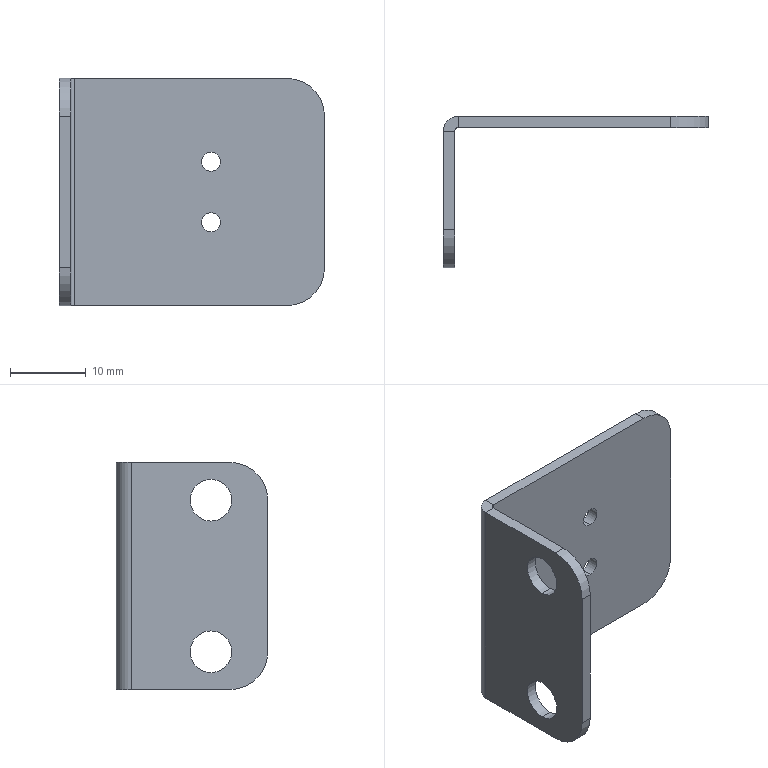Part | STEP file | 1 solid | 26 faces | box 35 x 20 x 30 mm | volume 2265 mm3 | cylinder 14 | plane 12 | commonest cylinder face diameters 2.5 x4 5.5 x4 10 x4 1 x1 4 x1